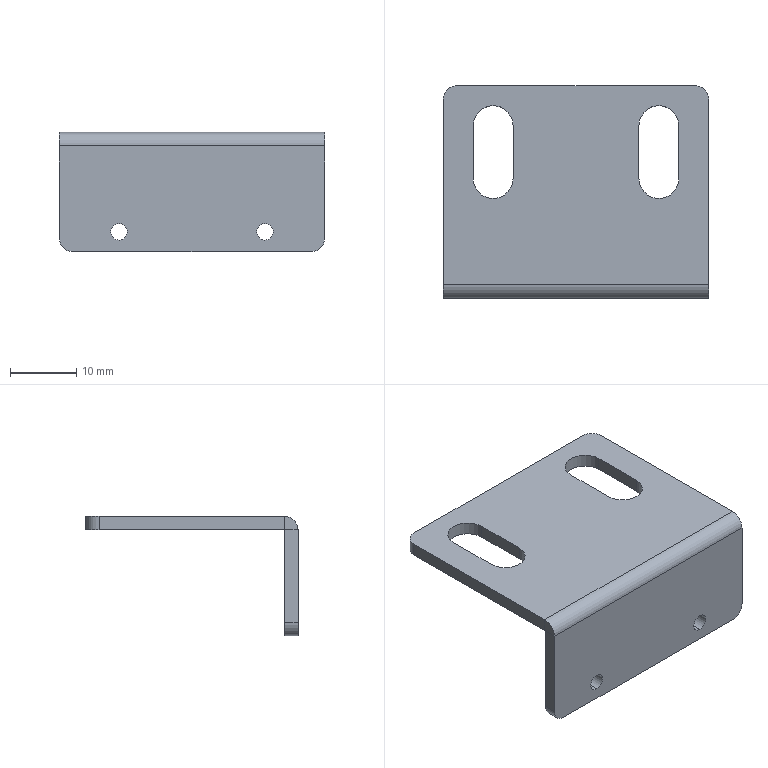Part | STEP file | proximity switch mounting plate 2 | 1 solid | 30 faces | box 40 x 32 x 18 mm | volume 3472 mm3 | plane 16 | cylinder 14 | commonest cylinder face diameters 2.5 x4 4 x4 6 x4 0.1 x1 4.1 x1